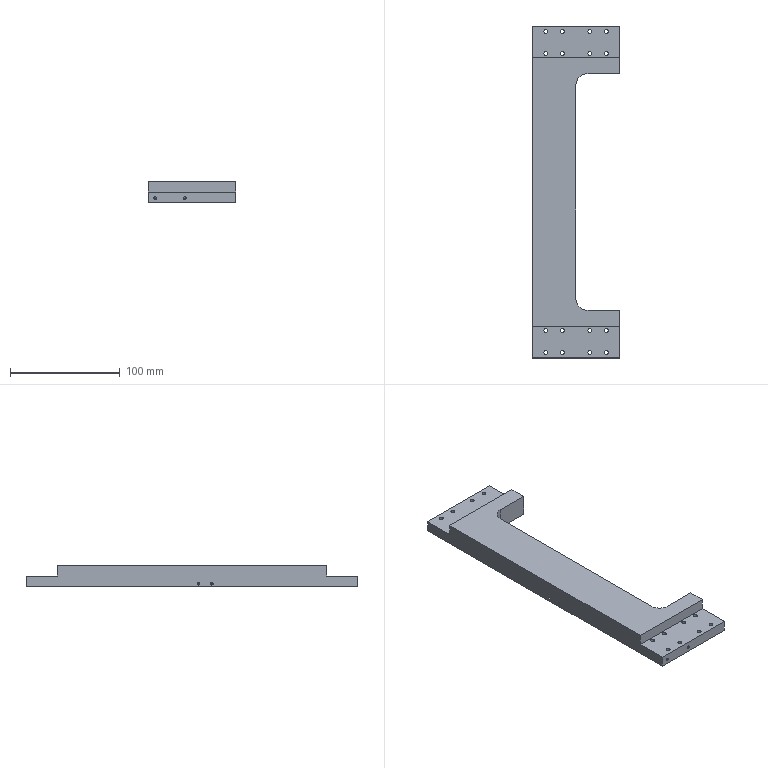Part | SolidWorks | features BaseBody 1 | 1 solid | 152 faces | box 80 x 302 x 20 mm | volume 261763 mm3 | cylinder 94 | plane 30 | cone 28 | commonest cylinder face diameters 3.5 x32 6 x32 4.134 x16 2.459 x12 20 x2